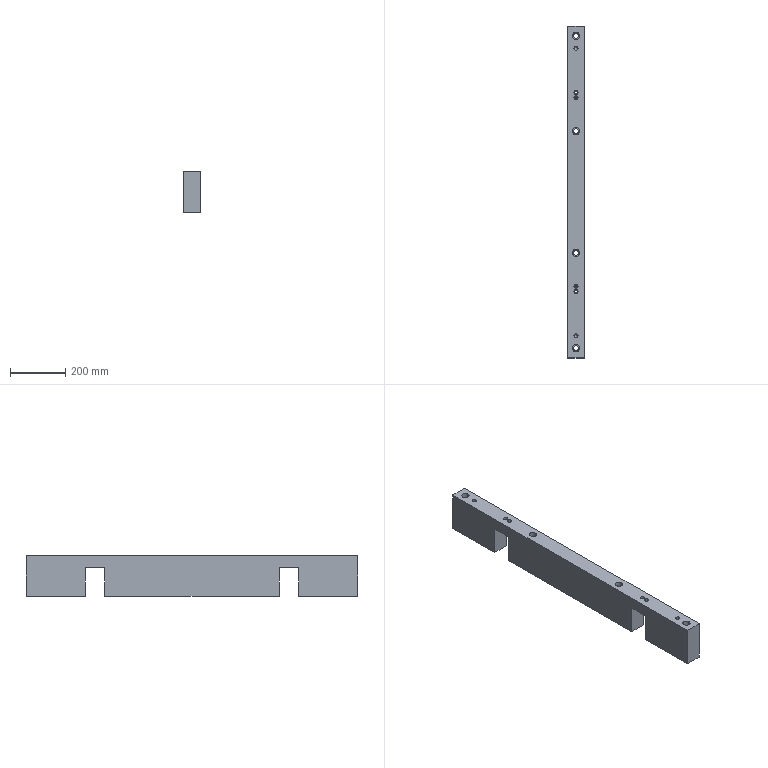Part | STEP file | lll_id2326_x_t | 1 solid | 42 faces | box 60 x 1200 x 147.5 mm | volume 9435645 mm3 | plane 22 | cylinder 18 | cone 2 | commonest cylinder face diameters 9.009 x4 14.508 x4 18.009 x4 26.008 x4 14.506 x2
STEP:
#1=CARTESIAN_POINT('',(2957.254,-340.,370.));
#2=VERTEX_POINT('',#1);
#3=CARTESIAN_POINT('',(2950.,-340.,370.));
#4=DIRECTION('',(0.,0.,-1.));
#5=DIRECTION('',(1.,0.,0.));
#6=AXIS2_PLACEMENT_3D('',#3,#4,#5);
#7=CIRCLE('',#6,7.254);
#8=EDGE_CURVE('',#2,#2,#7,.T.);
#9=ORIENTED_EDGE('',*,*,#8,.T.);
#10=EDGE_LOOP('',(#9));
#11=FACE_BOUND('',#10,.T.);
#12=CARTESIAN_POINT('',(2957.254,-360.,370.));
#13=VERTEX_POINT('',#12);
#14=CARTESIAN_POINT('',(2950.,-360.,370.));
#15=DIRECTION('',(0.,0.,-1.));
#16=DIRECTION('',(1.,0.,0.));
#17=AXIS2_PLACEMENT_3D('',#14,#15,#16);
#18=CIRCLE('',#17,7.254);
#19=EDGE_CURVE('',#13,#13,#18,.T.);
#20=ORIENTED_EDGE('',*,*,#19,.T.);
#21=EDGE_LOOP('',(#20));
#22=FACE_BOUND('',#21,.T.);
#23=CARTESIAN_POINT('',(2957.254,340.,370.));
#24=VERTEX_POINT('',#23);
#25=CARTESIAN_POINT('',(2950.,340.,370.));
#26=DIRECTION('',(0.,0.,-1.));
#27=DIRECTION('',(1.,0.,0.));
#28=AXIS2_PLACEMENT_3D('',#25,#26,#27);
#29=CIRCLE('',#28,7.254);
#30=EDGE_CURVE('',#24,#24,#29,.T.);
#31=ORIENTED_EDGE('',*,*,#30,.T.);
#32=EDGE_LOOP('',(#31));
#33=FACE_BOUND('',#32,.T.);
#34=CARTESIAN_POINT('',(2957.254,360.,370.));
#35=VERTEX_POINT('',#34);
#36=CARTESIAN_POINT('',(2950.,360.,370.));
#37=DIRECTION('',(0.,0.,-1.));
#38=DIRECTION('',(1.,0.,0.));
#39=AXIS2_PLACEMENT_3D('',#36,#37,#38);
#40=CIRCLE('',#39,7.254);
#41=EDGE_CURVE('',#35,#35,#40,.T.);
#42=ORIENTED_EDGE('',*,*,#41,.T.);
#43=EDGE_LOOP('',(#42));
#44=FACE_BOUND('',#43,.T.);
#45=CARTESIAN_POINT('',(2963.004,220.,370.));
#46=VERTEX_POINT('',#45);
#47=CARTESIAN_POINT('',(2950.,220.,370.));
#48=DIRECTION('',(0.,0.,1.));
#49=DIRECTION('',(1.,0.,0.));
#50=AXIS2_PLACEMENT_3D('',#47,#48,#49);
#51=CIRCLE('',#50,13.004);
#52=EDGE_CURVE('',#46,#46,#51,.T.);
#53=ORIENTED_EDGE('',*,*,#52,.F.);
#54=EDGE_LOOP('',(#53));
#55=FACE_BOUND('',#54,.T.);
#56=CARTESIAN_POINT('',(2963.004,-220.,370.));
#57=VERTEX_POINT('',#56);
#58=CARTESIAN_POINT('',(2950.,-220.,370.));
#59=DIRECTION('',(0.,0.,-1.));
#60=DIRECTION('',(1.,0.,0.));
#61=AXIS2_PLACEMENT_3D('',#58,#59,#60);
#62=CIRCLE('',#61,13.004);
#63=EDGE_CURVE('',#57,#57,#62,.T.);
#64=ORIENTED_EDGE('',*,*,#63,.T.);
#65=EDGE_LOOP('',(#64));
#66=FACE_BOUND('',#65,.T.);
#67=CARTESIAN_POINT('',(2963.004,-565.,370.));
#68=VERTEX_POINT('',#67);
#69=CARTESIAN_POINT('',(2950.,-565.,370.));
#70=DIRECTION('',(0.,0.,-1.));
#71=DIRECTION('',(1.,0.,0.));
#72=AXIS2_PLACEMENT_3D('',#69,#70,#71);
#73=CIRCLE('',#72,13.004);
#74=EDGE_CURVE('',#68,#68,#73,.T.);
#75=ORIENTED_EDGE('',*,*,#74,.T.);
#76=EDGE_LOOP('',(#75));
#77=FACE_BOUND('',#76,.T.);
#78=CARTESIAN_POINT('',(2980.,600.,370.));
#79=VERTEX_POINT('',#78);
#80=CARTESIAN_POINT('',(2920.,600.,370.));
#81=VERTEX_POINT('',#80);
#82=CARTESIAN_POINT('',(6890.,600.,370.));
#83=DIRECTION('',(-1.,0.,0.));
#84=VECTOR('',#83,1.);
#85=LINE('',#82,#84);
#86=EDGE_CURVE('',#79,#81,#85,.T.);
#87=ORIENTED_EDGE('',*,*,#86,.T.);
#88=CARTESIAN_POINT('',(2920.,-600.,370.));
#89=VERTEX_POINT('',#88);
#90=CARTESIAN_POINT('',(2920.,600.,370.));
#91=DIRECTION('',(0.,-1.,0.));
#92=VECTOR('',#91,1.);
#93=LINE('',#90,#92);
#94=EDGE_CURVE('',#81,#89,#93,.T.);
#95=ORIENTED_EDGE('',*,*,#94,.T.);
#96=CARTESIAN_POINT('',(2980.,-600.,370.));
#97=VERTEX_POINT('',#96);
#98=CARTESIAN_POINT('',(2920.,-600.,370.));
#99=DIRECTION('',(1.,0.,0.));
#100=VECTOR('',#99,1.);
#101=LINE('',#98,#100);
#102=EDGE_CURVE('',#89,#97,#101,.T.);
#103=ORIENTED_EDGE('',*,*,#102,.T.);
#104=CARTESIAN_POINT('',(2980.,1.,370.));
#105=DIRECTION('',(0.,1.,0.));
#106=VECTOR('',#105,1.);
#107=LINE('',#104,#106);
#108=EDGE_CURVE('',#97,#79,#107,.T.);
#109=ORIENTED_EDGE('',*,*,#108,.T.);
#110=EDGE_LOOP('',(#87,#95,#103,#109));
#111=FACE_BOUND('',#110,.T.);
#112=CARTESIAN_POINT('',(2963.004,565.,370.));
#113=VERTEX_POINT('',#112);
#114=CARTESIAN_POINT('',(2950.,565.,370.));
#115=DIRECTION('',(0.,0.,1.));
#116=DIRECTION('',(1.,0.,0.));
#117=AXIS2_PLACEMENT_3D('',#114,#115,#116);
#118=CIRCLE('',#117,13.004);
#119=EDGE_CURVE('',#113,#113,#118,.T.);
#120=ORIENTED_EDGE('',*,*,#119,.F.);
#121=EDGE_LOOP('',(#120));
#122=FACE_BOUND('',#121,.T.);
#123=CARTESIAN_POINT('',(2957.253,-520.,370.));
#124=VERTEX_POINT('',#123);
#125=CARTESIAN_POINT('',(2950.,-520.,370.));
#126=DIRECTION('',(0.,0.,-1.));
#127=DIRECTION('',(1.,0.,0.));
#128=AXIS2_PLACEMENT_3D('',#125,#126,#127);
#129=CIRCLE('',#128,7.253);
#130=EDGE_CURVE('',#124,#124,#129,.T.);
#131=ORIENTED_EDGE('',*,*,#130,.T.);
#132=EDGE_LOOP('',(#131));
#133=FACE_BOUND('',#132,.T.);
#134=CARTESIAN_POINT('',(2957.253,520.,370.));
#135=VERTEX_POINT('',#134);
#136=CARTESIAN_POINT('',(2950.,520.,370.));
#137=DIRECTION('',(0.,0.,1.));
#138=DIRECTION('',(1.,0.,0.));
#139=AXIS2_PLACEMENT_3D('',#136,#137,#138);
#140=CIRCLE('',#139,7.253);
#141=EDGE_CURVE('',#135,#135,#140,.T.);
#142=ORIENTED_EDGE('',*,*,#141,.F.);
#143=EDGE_LOOP('',(#142));
#144=FACE_BOUND('',#143,.T.);
#145=CARTESIAN_POINT('',(733.685,1.,370.));
#146=DIRECTION('',(0.,0.,-1.));
#147=DIRECTION('',(1.,0.,0.));
#148=AXIS2_PLACEMENT_3D('',#145,#146,#147);
#149=PLANE('',#148);
#150=ADVANCED_FACE('',(#11,#22,#33,#44,#55,#66,#77,#111,#122,#133,#144),#149,.F.);
#151=CARTESIAN_POINT('',(2980.,315.249,222.5));
#152=VERTEX_POINT('',#151);
#153=CARTESIAN_POINT('',(2920.,315.249,222.5));
#154=VERTEX_POINT('',#153);
#155=CARTESIAN_POINT('',(733.685,315.249,222.5));
#156=DIRECTION('',(-1.,0.,0.));
#157=VECTOR('',#156,1.);
#158=LINE('',#155,#157);
#159=EDGE_CURVE('',#152,#154,#158,.T.);
#160=ORIENTED_EDGE('',*,*,#159,.F.);
#161=CARTESIAN_POINT('',(2980.,-315.249,222.5));
#162=VERTEX_POINT('',#161);
#163=CARTESIAN_POINT('',(2980.,1.,222.5));
#164=DIRECTION('',(0.,-1.,0.));
#165=VECTOR('',#164,1.);
#166=LINE('',#163,#165);
#167=EDGE_CURVE('',#152,#162,#166,.T.);
#168=ORIENTED_EDGE('',*,*,#167,.T.);
#169=CARTESIAN_POINT('',(2920.,-315.249,222.5));
#170=VERTEX_POINT('',#169);
#171=CARTESIAN_POINT('',(733.685,-315.249,222.5));
#172=DIRECTION('',(1.,0.,0.));
#173=VECTOR('',#172,1.);
#174=LINE('',#171,#173);
#175=EDGE_CURVE('',#170,#162,#174,.T.);
#176=ORIENTED_EDGE('',*,*,#175,.F.);
#177=CARTESIAN_POINT('',(2920.,600.,222.5));
#178=DIRECTION('',(0.,-1.,0.));
#179=VECTOR('',#178,1.);
#180=LINE('',#177,#179);
#181=EDGE_CURVE('',#154,#170,#180,.T.);
#182=ORIENTED_EDGE('',*,*,#181,.F.);
#183=EDGE_LOOP('',(#160,#168,#176,#182));
#184=FACE_BOUND('',#183,.T.);
#185=CARTESIAN_POINT('',(2959.005,220.,222.5));
#186=VERTEX_POINT('',#185);
#187=CARTESIAN_POINT('',(2950.,220.,222.5));
#188=DIRECTION('',(0.,0.,-1.));
#189=DIRECTION('',(1.,0.,0.));
#190=AXIS2_PLACEMENT_3D('',#187,#188,#189);
#191=CIRCLE('',#190,9.005);
#192=EDGE_CURVE('',#186,#186,#191,.T.);
#193=ORIENTED_EDGE('',*,*,#192,.F.);
#194=EDGE_LOOP('',(#193));
#195=FACE_BOUND('',#194,.T.);
#196=CARTESIAN_POINT('',(2959.005,-220.,222.5));
#197=VERTEX_POINT('',#196);
#198=CARTESIAN_POINT('',(2950.,-220.,222.5));
#199=DIRECTION('',(0.,0.,1.));
#200=DIRECTION('',(1.,0.,0.));
#201=AXIS2_PLACEMENT_3D('',#198,#199,#200);
#202=CIRCLE('',#201,9.005);
#203=EDGE_CURVE('',#197,#197,#202,.T.);
#204=ORIENTED_EDGE('',*,*,#203,.T.);
#205=EDGE_LOOP('',(#204));
#206=FACE_BOUND('',#205,.T.);
#207=CARTESIAN_POINT('',(733.685,1.,222.5));
#208=DIRECTION('',(0.,0.,-1.));
#209=DIRECTION('',(1.,0.,0.));
#210=AXIS2_PLACEMENT_3D('',#207,#208,#209);
#211=PLANE('',#210);
#212=ADVANCED_FACE('',(#184,#195,#206),#211,.T.);
#213=CARTESIAN_POINT('',(2920.,385.249,222.5));
#214=VERTEX_POINT('',#213);
#215=CARTESIAN_POINT('',(2980.,385.249,222.5));
#216=VERTEX_POINT('',#215);
#217=CARTESIAN_POINT('',(733.685,385.249,222.5));
#218=DIRECTION('',(1.,0.,0.));
#219=VECTOR('',#218,1.);
#220=LINE('',#217,#219);
#221=EDGE_CURVE('',#214,#216,#220,.T.);
#222=ORIENTED_EDGE('',*,*,#221,.F.);
#223=CARTESIAN_POINT('',(2920.,600.,222.5));
#224=VERTEX_POINT('',#223);
#225=CARTESIAN_POINT('',(2920.,600.,222.5));
#226=DIRECTION('',(0.,-1.,0.));
#227=VECTOR('',#226,1.);
#228=LINE('',#225,#227);
#229=EDGE_CURVE('',#224,#214,#228,.T.);
#230=ORIENTED_EDGE('',*,*,#229,.F.);
#231=CARTESIAN_POINT('',(2980.,600.,222.5));
#232=VERTEX_POINT('',#231);
#233=CARTESIAN_POINT('',(6890.,600.,222.5));
#234=DIRECTION('',(-1.,0.,0.));
#235=VECTOR('',#234,1.);
#236=LINE('',#233,#235);
#237=EDGE_CURVE('',#232,#224,#236,.T.);
#238=ORIENTED_EDGE('',*,*,#237,.F.);
#239=CARTESIAN_POINT('',(2980.,1.,222.5));
#240=DIRECTION('',(0.,-1.,0.));
#241=VECTOR('',#240,1.);
#242=LINE('',#239,#241);
#243=EDGE_CURVE('',#232,#216,#242,.T.);
#244=ORIENTED_EDGE('',*,*,#243,.T.);
#245=EDGE_LOOP('',(#222,#230,#238,#244));
#246=FACE_BOUND('',#245,.T.);
#247=CARTESIAN_POINT('',(2959.005,565.,222.5));
#248=VERTEX_POINT('',#247);
#249=CARTESIAN_POINT('',(2950.,565.,222.5));
#250=DIRECTION('',(0.,0.,-1.));
#251=DIRECTION('',(1.,0.,0.));
#252=AXIS2_PLACEMENT_3D('',#249,#250,#251);
#253=CIRCLE('',#252,9.005);
#254=EDGE_CURVE('',#248,#248,#253,.T.);
#255=ORIENTED_EDGE('',*,*,#254,.F.);
#256=EDGE_LOOP('',(#255));
#257=FACE_BOUND('',#256,.T.);
#258=CARTESIAN_POINT('',(733.685,1.,222.5));
#259=DIRECTION('',(0.,0.,-1.));
#260=DIRECTION('',(1.,0.,0.));
#261=AXIS2_PLACEMENT_3D('',#258,#259,#260);
#262=PLANE('',#261);
#263=ADVANCED_FACE('',(#246,#257),#262,.T.);
#264=CARTESIAN_POINT('',(2980.,-385.249,222.5));
#265=VERTEX_POINT('',#264);
#266=CARTESIAN_POINT('',(2920.,-385.249,222.5));
#267=VERTEX_POINT('',#266);
#268=CARTESIAN_POINT('',(733.685,-385.249,222.5));
#269=DIRECTION('',(-1.,0.,0.));
#270=VECTOR('',#269,1.);
#271=LINE('',#268,#270);
#272=EDGE_CURVE('',#265,#267,#271,.T.);
#273=ORIENTED_EDGE('',*,*,#272,.F.);
#274=CARTESIAN_POINT('',(2980.,-600.,222.5));
#275=VERTEX_POINT('',#274);
#276=CARTESIAN_POINT('',(2980.,1.,222.5));
#277=DIRECTION('',(0.,-1.,0.));
#278=VECTOR('',#277,1.);
#279=LINE('',#276,#278);
#280=EDGE_CURVE('',#265,#275,#279,.T.);
#281=ORIENTED_EDGE('',*,*,#280,.T.);
#282=CARTESIAN_POINT('',(2920.,-600.,222.5));
#283=VERTEX_POINT('',#282);
#284=CARTESIAN_POINT('',(2920.,-600.,222.5));
#285=DIRECTION('',(1.,0.,0.));
#286=VECTOR('',#285,1.);
#287=LINE('',#284,#286);
#288=EDGE_CURVE('',#283,#275,#287,.T.);
#289=ORIENTED_EDGE('',*,*,#288,.F.);
#290=CARTESIAN_POINT('',(2920.,600.,222.5));
#291=DIRECTION('',(0.,-1.,0.));
#292=VECTOR('',#291,1.);
#293=LINE('',#290,#292);
#294=EDGE_CURVE('',#267,#283,#293,.T.);
#295=ORIENTED_EDGE('',*,*,#294,.F.);
#296=EDGE_LOOP('',(#273,#281,#289,#295));
#297=FACE_BOUND('',#296,.T.);
#298=CARTESIAN_POINT('',(2959.005,-565.,222.5));
#299=VERTEX_POINT('',#298);
#300=CARTESIAN_POINT('',(2950.,-565.,222.5));
#301=DIRECTION('',(0.,0.,1.));
#302=DIRECTION('',(1.,0.,0.));
#303=AXIS2_PLACEMENT_3D('',#300,#301,#302);
#304=CIRCLE('',#303,9.005);
#305=EDGE_CURVE('',#299,#299,#304,.T.);
#306=ORIENTED_EDGE('',*,*,#305,.T.);
#307=EDGE_LOOP('',(#306));
#308=FACE_BOUND('',#307,.T.);
#309=CARTESIAN_POINT('',(733.685,1.,222.5));
#310=DIRECTION('',(0.,0.,-1.));
#311=DIRECTION('',(1.,0.,0.));
#312=AXIS2_PLACEMENT_3D('',#309,#310,#311);
#313=PLANE('',#312);
#314=ADVANCED_FACE('',(#297,#308),#313,.T.);
#315=CARTESIAN_POINT('',(2920.,315.249,326.5));
#316=VERTEX_POINT('',#315);
#317=CARTESIAN_POINT('',(2920.,315.249,310.));
#318=DIRECTION('',(0.,0.,1.));
#319=VECTOR('',#318,1.);
#320=LINE('',#317,#319);
#321=EDGE_CURVE('',#154,#316,#320,.T.);
#322=ORIENTED_EDGE('',*,*,#321,.F.);
#323=ORIENTED_EDGE('',*,*,#181,.T.);
#324=CARTESIAN_POINT('',(2920.,-315.249,326.5));
#325=VERTEX_POINT('',#324);
#326=CARTESIAN_POINT('',(2920.,-315.249,310.));
#327=DIRECTION('',(0.,0.,-1.));
#328=VECTOR('',#327,1.);
#329=LINE('',#326,#328);
#330=EDGE_CURVE('',#325,#170,#329,.T.);
#331=ORIENTED_EDGE('',*,*,#330,.F.);
#332=CARTESIAN_POINT('',(2920.,-385.249,326.5));
#333=VERTEX_POINT('',#332);
#334=CARTESIAN_POINT('',(2920.,600.,326.5));
#335=DIRECTION('',(0.,1.,0.));
#336=VECTOR('',#335,1.);
#337=LINE('',#334,#336);
#338=EDGE_CURVE('',#333,#325,#337,.T.);
#339=ORIENTED_EDGE('',*,*,#338,.F.);
#340=CARTESIAN_POINT('',(2920.,-385.249,310.));
#341=DIRECTION('',(0.,0.,1.));
#342=VECTOR('',#341,1.);
#343=LINE('',#340,#342);
#344=EDGE_CURVE('',#267,#333,#343,.T.);
#345=ORIENTED_EDGE('',*,*,#344,.F.);
#346=ORIENTED_EDGE('',*,*,#294,.T.);
#347=CARTESIAN_POINT('',(2920.,-600.,310.));
#348=DIRECTION('',(0.,0.,-1.));
#349=VECTOR('',#348,1.);
#350=LINE('',#347,#349);
#351=EDGE_CURVE('',#89,#283,#350,.T.);
#352=ORIENTED_EDGE('',*,*,#351,.F.);
#353=ORIENTED_EDGE('',*,*,#94,.F.);
#354=CARTESIAN_POINT('',(2920.,600.,310.));
#355=DIRECTION('',(0.,0.,-1.));
#356=VECTOR('',#355,1.);
#357=LINE('',#354,#356);
#358=EDGE_CURVE('',#81,#224,#357,.T.);
#359=ORIENTED_EDGE('',*,*,#358,.T.);
#360=ORIENTED_EDGE('',*,*,#229,.T.);
#361=CARTESIAN_POINT('',(2920.,385.249,326.5));
#362=VERTEX_POINT('',#361);
#363=CARTESIAN_POINT('',(2920.,385.249,310.));
#364=DIRECTION('',(0.,0.,-1.));
#365=VECTOR('',#364,1.);
#366=LINE('',#363,#365);
#367=EDGE_CURVE('',#362,#214,#366,.T.);
#368=ORIENTED_EDGE('',*,*,#367,.F.);
#369=CARTESIAN_POINT('',(2920.,600.,326.5));
#370=DIRECTION('',(0.,1.,0.));
#371=VECTOR('',#370,1.);
#372=LINE('',#369,#371);
#373=EDGE_CURVE('',#316,#362,#372,.T.);
#374=ORIENTED_EDGE('',*,*,#373,.F.);
#375=EDGE_LOOP('',(#322,#323,#331,#339,#345,#346,#352,#353,#359,#360,#368,#374));
#376=FACE_OUTER_BOUND('',#375,.T.);
#377=CARTESIAN_POINT('',(2920.,600.,310.));
#378=DIRECTION('',(-1.,0.,0.));
#379=DIRECTION('',(0.,0.,-1.));
#380=AXIS2_PLACEMENT_3D('',#377,#378,#379);
#381=PLANE('',#380);
#382=ADVANCED_FACE('',(#376),#381,.T.);
#383=CARTESIAN_POINT('',(2980.,-600.,310.));
#384=DIRECTION('',(0.,0.,-1.));
#385=VECTOR('',#384,1.);
#386=LINE('',#383,#385);
#387=EDGE_CURVE('',#97,#275,#386,.T.);
#388=ORIENTED_EDGE('',*,*,#387,.F.);
#389=ORIENTED_EDGE('',*,*,#102,.F.);
#390=ORIENTED_EDGE('',*,*,#351,.T.);
#391=ORIENTED_EDGE('',*,*,#288,.T.);
#392=EDGE_LOOP('',(#388,#389,#390,#391));
#393=FACE_OUTER_BOUND('',#392,.T.);
#394=CARTESIAN_POINT('',(2920.,-600.,310.));
#395=DIRECTION('',(0.,-1.,0.));
#396=DIRECTION('',(0.,0.,-1.));
#397=AXIS2_PLACEMENT_3D('',#394,#395,#396);
#398=PLANE('',#397);
#399=ADVANCED_FACE('',(#393),#398,.T.);
#400=CARTESIAN_POINT('',(2980.,600.,310.));
#401=DIRECTION('',(0.,0.,1.));
#402=VECTOR('',#401,1.);
#403=LINE('',#400,#402);
#404=EDGE_CURVE('',#232,#79,#403,.T.);
#405=ORIENTED_EDGE('',*,*,#404,.F.);
#406=ORIENTED_EDGE('',*,*,#237,.T.);
#407=ORIENTED_EDGE('',*,*,#358,.F.);
#408=ORIENTED_EDGE('',*,*,#86,.F.);
#409=EDGE_LOOP('',(#405,#406,#407,#408));
#410=FACE_OUTER_BOUND('',#409,.T.);
#411=CARTESIAN_POINT('',(6890.,600.,310.));
#412=DIRECTION('',(0.,1.,0.));
#413=DIRECTION('',(0.,0.,1.));
#414=AXIS2_PLACEMENT_3D('',#411,#412,#413);
#415=PLANE('',#414);
#416=ADVANCED_FACE('',(#410),#415,.T.);
#417=ORIENTED_EDGE('',*,*,#167,.F.);
#418=CARTESIAN_POINT('',(2980.,315.249,326.5));
#419=VERTEX_POINT('',#418);
#420=CARTESIAN_POINT('',(2980.,315.249,241.25));
#421=DIRECTION('',(0.,0.,1.));
#422=VECTOR('',#421,1.);
#423=LINE('',#420,#422);
#424=EDGE_CURVE('',#152,#419,#423,.T.);
#425=ORIENTED_EDGE('',*,*,#424,.T.);
#426=CARTESIAN_POINT('',(2980.,385.249,326.5));
#427=VERTEX_POINT('',#426);
#428=CARTESIAN_POINT('',(2980.,0.,326.5));
#429=DIRECTION('',(0.,1.,0.));
#430=VECTOR('',#429,1.);
#431=LINE('',#428,#430);
#432=EDGE_CURVE('',#419,#427,#431,.T.);
#433=ORIENTED_EDGE('',*,*,#432,.T.);
#434=CARTESIAN_POINT('',(2980.,385.249,241.25));
#435=DIRECTION('',(0.,0.,-1.));
#436=VECTOR('',#435,1.);
#437=LINE('',#434,#436);
#438=EDGE_CURVE('',#427,#216,#437,.T.);
#439=ORIENTED_EDGE('',*,*,#438,.T.);
#440=ORIENTED_EDGE('',*,*,#243,.F.);
#441=ORIENTED_EDGE('',*,*,#404,.T.);
#442=ORIENTED_EDGE('',*,*,#108,.F.);
#443=ORIENTED_EDGE('',*,*,#387,.T.);
#444=ORIENTED_EDGE('',*,*,#280,.F.);
#445=CARTESIAN_POINT('',(2980.,-385.249,326.5));
#446=VERTEX_POINT('',#445);
#447=CARTESIAN_POINT('',(2980.,-385.249,241.25));
#448=DIRECTION('',(0.,0.,1.));
#449=VECTOR('',#448,1.);
#450=LINE('',#447,#449);
#451=EDGE_CURVE('',#265,#446,#450,.T.);
#452=ORIENTED_EDGE('',*,*,#451,.T.);
#453=CARTESIAN_POINT('',(2980.,-315.249,326.5));
#454=VERTEX_POINT('',#453);
#455=CARTESIAN_POINT('',(2980.,0.,326.5));
#456=DIRECTION('',(0.,1.,0.));
#457=VECTOR('',#456,1.);
#458=LINE('',#455,#457);
#459=EDGE_CURVE('',#446,#454,#458,.T.);
#460=ORIENTED_EDGE('',*,*,#459,.T.);
#461=CARTESIAN_POINT('',(2980.,-315.249,241.25));
#462=DIRECTION('',(0.,0.,-1.));
#463=VECTOR('',#462,1.);
#464=LINE('',#461,#463);
#465=EDGE_CURVE('',#454,#162,#464,.T.);
#466=ORIENTED_EDGE('',*,*,#465,.T.);
#467=EDGE_LOOP('',(#417,#425,#433,#439,#440,#441,#442,#443,#444,#452,#460,#466));
#468=FACE_OUTER_BOUND('',#467,.T.);
#469=CARTESIAN_POINT('',(2980.,0.,241.25));
#470=DIRECTION('',(-1.,0.,0.));
#471=DIRECTION('',(0.,0.,-1.));
#472=AXIS2_PLACEMENT_3D('',#469,#470,#471);
#473=PLANE('',#472);
#474=ADVANCED_FACE('',(#468),#473,.F.);
#475=CARTESIAN_POINT('',(2940.995,-565.,251.));
#476=VERTEX_POINT('',#475);
#477=CARTESIAN_POINT('',(2950.,-565.,251.));
#478=DIRECTION('',(0.,0.,-1.));
#479=DIRECTION('',(-1.,0.,0.));
#480=AXIS2_PLACEMENT_3D('',#477,#478,#479);
#481=CIRCLE('',#480,9.005);
#482=EDGE_CURVE('',#476,#476,#481,.T.);
#483=ORIENTED_EDGE('',*,*,#482,.F.);
#484=EDGE_LOOP('',(#483));
#485=FACE_BOUND('',#484,.T.);
#486=ORIENTED_EDGE('',*,*,#305,.F.);
#487=EDGE_LOOP('',(#486));
#488=FACE_BOUND('',#487,.T.);
#489=CARTESIAN_POINT('',(2950.,-565.,370.));
#490=DIRECTION('',(0.,0.,-1.));
#491=DIRECTION('',(1.,0.,0.));
#492=AXIS2_PLACEMENT_3D('',#489,#490,#491);
#493=CYLINDRICAL_SURFACE('',#492,9.005);
#494=ADVANCED_FACE('',(#485,#488),#493,.F.);
#495=ORIENTED_EDGE('',*,*,#482,.T.);
#496=EDGE_LOOP('',(#495));
#497=FACE_BOUND('',#496,.T.);
#498=CARTESIAN_POINT('',(2963.004,-565.,251.));
#499=VERTEX_POINT('',#498);
#500=CARTESIAN_POINT('',(2950.,-565.,251.));
#501=DIRECTION('',(0.,0.,-1.));
#502=DIRECTION('',(1.,0.,0.));
#503=AXIS2_PLACEMENT_3D('',#500,#501,#502);
#504=CIRCLE('',#503,13.004);
#505=EDGE_CURVE('',#499,#499,#504,.T.);
#506=ORIENTED_EDGE('',*,*,#505,.F.);
#507=EDGE_LOOP('',(#506));
#508=FACE_BOUND('',#507,.T.);
#509=CARTESIAN_POINT('',(2950.,-565.,251.));
#510=DIRECTION('',(0.,0.,-1.));
#511=DIRECTION('',(-1.,0.,0.));
#512=AXIS2_PLACEMENT_3D('',#509,#510,#511);
#513=PLANE('',#512);
#514=ADVANCED_FACE('',(#497,#508),#513,.F.);
#515=ORIENTED_EDGE('',*,*,#505,.T.);
#516=EDGE_LOOP('',(#515));
#517=FACE_BOUND('',#516,.T.);
#518=ORIENTED_EDGE('',*,*,#74,.F.);
#519=EDGE_LOOP('',(#518));
#520=FACE_BOUND('',#519,.T.);
#521=CARTESIAN_POINT('',(2950.,-565.,370.));
#522=DIRECTION('',(0.,0.,-1.));
#523=DIRECTION('',(1.,0.,0.));
#524=AXIS2_PLACEMENT_3D('',#521,#522,#523);
#525=CYLINDRICAL_SURFACE('',#524,13.004);
#526=ADVANCED_FACE('',(#517,#520),#525,.F.);
#527=CARTESIAN_POINT('',(2940.995,-220.,251.));
#528=VERTEX_POINT('',#527);
#529=CARTESIAN_POINT('',(2950.,-220.,251.));
#530=DIRECTION('',(0.,0.,-1.));
#531=DIRECTION('',(-1.,0.,0.));
#532=AXIS2_PLACEMENT_3D('',#529,#530,#531);
#533=CIRCLE('',#532,9.005);
#534=EDGE_CURVE('',#528,#528,#533,.T.);
#535=ORIENTED_EDGE('',*,*,#534,.F.);
#536=EDGE_LOOP('',(#535));
#537=FACE_BOUND('',#536,.T.);
#538=ORIENTED_EDGE('',*,*,#203,.F.);
#539=EDGE_LOOP('',(#538));
#540=FACE_BOUND('',#539,.T.);
#541=CARTESIAN_POINT('',(2950.,-220.,370.));
#542=DIRECTION('',(0.,0.,-1.));
#543=DIRECTION('',(1.,0.,0.));
#544=AXIS2_PLACEMENT_3D('',#541,#542,#543);
#545=CYLINDRICAL_SURFACE('',#544,9.005);
#546=ADVANCED_FACE('',(#537,#540),#545,.F.);
#547=ORIENTED_EDGE('',*,*,#534,.T.);
#548=EDGE_LOOP('',(#547));
#549=FACE_BOUND('',#548,.T.);
#550=CARTESIAN_POINT('',(2963.004,-220.,251.));
#551=VERTEX_POINT('',#550);
#552=CARTESIAN_POINT('',(2950.,-220.,251.));
#553=DIRECTION('',(0.,0.,-1.));
#554=DIRECTION('',(1.,0.,0.));
#555=AXIS2_PLACEMENT_3D('',#552,#553,#554);
#556=CIRCLE('',#555,13.004);
#557=EDGE_CURVE('',#551,#551,#556,.T.);
#558=ORIENTED_EDGE('',*,*,#557,.F.);
#559=EDGE_LOOP('',(#558));
#560=FACE_BOUND('',#559,.T.);
#561=CARTESIAN_POINT('',(2950.,-220.,251.));
#562=DIRECTION('',(0.,0.,-1.));
#563=DIRECTION('',(-1.,0.,0.));
#564=AXIS2_PLACEMENT_3D('',#561,#562,#563);
#565=PLANE('',#564);
#566=ADVANCED_FACE('',(#549,#560),#565,.F.);
#567=ORIENTED_EDGE('',*,*,#557,.T.);
#568=EDGE_LOOP('',(#567));
#569=FACE_BOUND('',#568,.T.);
#570=ORIENTED_EDGE('',*,*,#63,.F.);
#571=EDGE_LOOP('',(#570));
#572=FACE_BOUND('',#571,.T.);
#573=CARTESIAN_POINT('',(2950.,-220.,370.));
#574=DIRECTION('',(0.,0.,-1.));
#575=DIRECTION('',(1.,0.,0.));
#576=AXIS2_PLACEMENT_3D('',#573,#574,#575);
#577=CYLINDRICAL_SURFACE('',#576,13.004);
#578=ADVANCED_FACE('',(#569,#572),#577,.F.);
#579=CARTESIAN_POINT('',(2940.995,220.,251.));
#580=VERTEX_POINT('',#579);
#581=CARTESIAN_POINT('',(2950.,220.,251.));
#582=DIRECTION('',(0.,0.,1.));
#583=DIRECTION('',(-1.,0.,0.));
#584=AXIS2_PLACEMENT_3D('',#581,#582,#583);
#585=CIRCLE('',#584,9.005);
#586=EDGE_CURVE('',#580,#580,#585,.T.);
#587=ORIENTED_EDGE('',*,*,#586,.T.);
#588=EDGE_LOOP('',(#587));
#589=FACE_BOUND('',#588,.T.);
#590=ORIENTED_EDGE('',*,*,#192,.T.);
#591=EDGE_LOOP('',(#590));
#592=FACE_BOUND('',#591,.T.);
#593=CARTESIAN_POINT('',(2950.,220.,370.));
#594=DIRECTION('',(0.,0.,-1.));
#595=DIRECTION('',(1.,0.,0.));
#596=AXIS2_PLACEMENT_3D('',#593,#594,#595);
#597=CYLINDRICAL_SURFACE('',#596,9.005);
#598=ADVANCED_FACE('',(#589,#592),#597,.F.);
#599=ORIENTED_EDGE('',*,*,#586,.F.);
#600=EDGE_LOOP('',(#599));
#601=FACE_BOUND('',#600,.T.);
#602=CARTESIAN_POINT('',(2963.004,220.,251.));
#603=VERTEX_POINT('',#602);
#604=CARTESIAN_POINT('',(2950.,220.,251.));
#605=DIRECTION('',(0.,0.,1.));
#606=DIRECTION('',(1.,0.,0.));
#607=AXIS2_PLACEMENT_3D('',#604,#605,#606);
#608=CIRCLE('',#607,13.004);
#609=EDGE_CURVE('',#603,#603,#608,.T.);
#610=ORIENTED_EDGE('',*,*,#609,.T.);
#611=EDGE_LOOP('',(#610));
#612=FACE_BOUND('',#611,.T.);
#613=CARTESIAN_POINT('',(2950.,220.,251.));
#614=DIRECTION('',(0.,0.,-1.));
#615=DIRECTION('',(-1.,0.,0.));
#616=AXIS2_PLACEMENT_3D('',#613,#614,#615);
#617=PLANE('',#616);
#618=ADVANCED_FACE('',(#601,#612),#617,.F.);
#619=ORIENTED_EDGE('',*,*,#609,.F.);
#620=EDGE_LOOP('',(#619));
#621=FACE_BOUND('',#620,.T.);
#622=ORIENTED_EDGE('',*,*,#52,.T.);
#623=EDGE_LOOP('',(#622));
#624=FACE_BOUND('',#623,.T.);
#625=CARTESIAN_POINT('',(2950.,220.,370.));
#626=DIRECTION('',(0.,0.,-1.));
#627=DIRECTION('',(1.,0.,0.));
#628=AXIS2_PLACEMENT_3D('',#625,#626,#627);
#629=CYLINDRICAL_SURFACE('',#628,13.004);
#630=ADVANCED_FACE('',(#621,#624),#629,.F.);
#631=CARTESIAN_POINT('',(2940.995,565.,251.));
#632=VERTEX_POINT('',#631);
#633=CARTESIAN_POINT('',(2950.,565.,251.));
#634=DIRECTION('',(0.,0.,1.));
#635=DIRECTION('',(-1.,0.,0.));
#636=AXIS2_PLACEMENT_3D('',#633,#634,#635);
#637=CIRCLE('',#636,9.005);
#638=EDGE_CURVE('',#632,#632,#637,.T.);
#639=ORIENTED_EDGE('',*,*,#638,.T.);
#640=EDGE_LOOP('',(#639));
#641=FACE_BOUND('',#640,.T.);
#642=ORIENTED_EDGE('',*,*,#254,.T.);
#643=EDGE_LOOP('',(#642));
#644=FACE_BOUND('',#643,.T.);
#645=CARTESIAN_POINT('',(2950.,565.,370.));
#646=DIRECTION('',(0.,0.,-1.));
#647=DIRECTION('',(1.,0.,0.));
#648=AXIS2_PLACEMENT_3D('',#645,#646,#647);
#649=CYLINDRICAL_SURFACE('',#648,9.005);
#650=ADVANCED_FACE('',(#641,#644),#649,.F.);
#651=ORIENTED_EDGE('',*,*,#638,.F.);
#652=EDGE_LOOP('',(#651));
#653=FACE_BOUND('',#652,.T.);
#654=CARTESIAN_POINT('',(2963.004,565.,251.));
#655=VERTEX_POINT('',#654);
#656=CARTESIAN_POINT('',(2950.,565.,251.));
#657=DIRECTION('',(0.,0.,1.));
#658=DIRECTION('',(1.,0.,0.));
#659=AXIS2_PLACEMENT_3D('',#656,#657,#658);
#660=CIRCLE('',#659,13.004);
#661=EDGE_CURVE('',#655,#655,#660,.T.);
#662=ORIENTED_EDGE('',*,*,#661,.T.);
#663=EDGE_LOOP('',(#662));
#664=FACE_BOUND('',#663,.T.);
#665=CARTESIAN_POINT('',(2950.,565.,251.));
#666=DIRECTION('',(0.,0.,-1.));
#667=DIRECTION('',(-1.,0.,0.));
#668=AXIS2_PLACEMENT_3D('',#665,#666,#667);
#669=PLANE('',#668);
#670=ADVANCED_FACE('',(#653,#664),#669,.F.);
#671=ORIENTED_EDGE('',*,*,#661,.F.);
#672=EDGE_LOOP('',(#671));
#673=FACE_BOUND('',#672,.T.);
#674=ORIENTED_EDGE('',*,*,#119,.T.);
#675=EDGE_LOOP('',(#674));
#676=FACE_BOUND('',#675,.T.);
#677=CARTESIAN_POINT('',(2950.,565.,370.));
#678=DIRECTION('',(0.,0.,-1.));
#679=DIRECTION('',(1.,0.,0.));
#680=AXIS2_PLACEMENT_3D('',#677,#678,#679);
#681=CYLINDRICAL_SURFACE('',#680,13.004);
#682=ADVANCED_FACE('',(#673,#676),#681,.F.);
#683=CARTESIAN_POINT('',(2954.505,-340.,326.5));
#684=VERTEX_POINT('',#683);
#685=CARTESIAN_POINT('',(2950.,-340.,326.5));
#686=DIRECTION('',(0.,0.,1.));
#687=DIRECTION('',(1.,0.,0.));
#688=AXIS2_PLACEMENT_3D('',#685,#686,#687);
#689=CIRCLE('',#688,4.505);
#690=EDGE_CURVE('',#684,#684,#689,.T.);
#691=ORIENTED_EDGE('',*,*,#690,.T.);
#692=EDGE_LOOP('',(#691));
#693=FACE_BOUND('',#692,.T.);
#694=CARTESIAN_POINT('',(2954.505,-360.,326.5));
#695=VERTEX_POINT('',#694);
#696=CARTESIAN_POINT('',(2950.,-360.,326.5));
#697=DIRECTION('',(0.,0.,1.));
#698=DIRECTION('',(1.,0.,0.));
#699=AXIS2_PLACEMENT_3D('',#696,#697,#698);
#700=CIRCLE('',#699,4.505);
#701=EDGE_CURVE('',#695,#695,#700,.T.);
#702=ORIENTED_EDGE('',*,*,#701,.T.);
#703=EDGE_LOOP('',(#702));
#704=FACE_BOUND('',#703,.T.);
#705=ORIENTED_EDGE('',*,*,#338,.T.);
#706=CARTESIAN_POINT('',(2950.,-315.249,326.5));
#707=DIRECTION('',(1.,0.,0.));
#708=VECTOR('',#707,1.);
#709=LINE('',#706,#708);
#710=EDGE_CURVE('',#325,#454,#709,.T.);
#711=ORIENTED_EDGE('',*,*,#710,.T.);
#712=ORIENTED_EDGE('',*,*,#459,.F.);
#713=CARTESIAN_POINT('',(2950.,-385.249,326.5));
#714=DIRECTION('',(-1.,0.,0.));
#715=VECTOR('',#714,1.);
#716=LINE('',#713,#715);
#717=EDGE_CURVE('',#446,#333,#716,.T.);
#718=ORIENTED_EDGE('',*,*,#717,.T.);
#719=EDGE_LOOP('',(#705,#711,#712,#718));
#720=FACE_BOUND('',#719,.T.);
#721=CARTESIAN_POINT('',(2950.,-350.249,326.5));
#722=DIRECTION('',(0.,0.,1.));
#723=DIRECTION('',(1.,0.,0.));
#724=AXIS2_PLACEMENT_3D('',#721,#722,#723);
#725=PLANE('',#724);
#726=ADVANCED_FACE('',(#693,#704,#720),#725,.F.);
#727=ORIENTED_EDGE('',*,*,#330,.T.);
#728=ORIENTED_EDGE('',*,*,#175,.T.);
#729=ORIENTED_EDGE('',*,*,#465,.F.);
#730=ORIENTED_EDGE('',*,*,#710,.F.);
#731=EDGE_LOOP('',(#727,#728,#729,#730));
#732=FACE_OUTER_BOUND('',#731,.T.);
#733=CARTESIAN_POINT('',(2950.,-315.249,76.5));
#734=DIRECTION('',(0.,1.,0.));
#735=DIRECTION('',(0.,0.,-1.));
#736=AXIS2_PLACEMENT_3D('',#733,#734,#735);
#737=PLANE('',#736);
#738=ADVANCED_FACE('',(#732),#737,.F.);
#739=ORIENTED_EDGE('',*,*,#344,.T.);
#740=ORIENTED_EDGE('',*,*,#717,.F.);
#741=ORIENTED_EDGE('',*,*,#451,.F.);
#742=ORIENTED_EDGE('',*,*,#272,.T.);
#743=EDGE_LOOP('',(#739,#740,#741,#742));
#744=FACE_OUTER_BOUND('',#743,.T.);
#745=CARTESIAN_POINT('',(2950.,-385.249,76.5));
#746=DIRECTION('',(0.,-1.,0.));
#747=DIRECTION('',(0.,0.,1.));
#748=AXIS2_PLACEMENT_3D('',#745,#746,#747);
#749=PLANE('',#748);
#750=ADVANCED_FACE('',(#744),#749,.F.);
#751=CARTESIAN_POINT('',(2954.505,340.,326.5));
#752=VERTEX_POINT('',#751);
#753=CARTESIAN_POINT('',(2950.,340.,326.5));
#754=DIRECTION('',(0.,0.,1.));
#755=DIRECTION('',(1.,0.,0.));
#756=AXIS2_PLACEMENT_3D('',#753,#754,#755);
#757=CIRCLE('',#756,4.505);
#758=EDGE_CURVE('',#752,#752,#757,.T.);
#759=ORIENTED_EDGE('',*,*,#758,.T.);
#760=EDGE_LOOP('',(#759));
#761=FACE_BOUND('',#760,.T.);
#762=CARTESIAN_POINT('',(2954.505,360.,326.5));
#763=VERTEX_POINT('',#762);
#764=CARTESIAN_POINT('',(2950.,360.,326.5));
#765=DIRECTION('',(0.,0.,1.));
#766=DIRECTION('',(1.,0.,0.));
#767=AXIS2_PLACEMENT_3D('',#764,#765,#766);
#768=CIRCLE('',#767,4.505);
#769=EDGE_CURVE('',#763,#763,#768,.T.);
#770=ORIENTED_EDGE('',*,*,#769,.T.);
#771=EDGE_LOOP('',(#770));
#772=FACE_BOUND('',#771,.T.);
#773=ORIENTED_EDGE('',*,*,#373,.T.);
#774=CARTESIAN_POINT('',(2950.,385.249,326.5));
#775=DIRECTION('',(-1.,0.,0.));
#776=VECTOR('',#775,1.);
#777=LINE('',#774,#776);
#778=EDGE_CURVE('',#427,#362,#777,.T.);
#779=ORIENTED_EDGE('',*,*,#778,.F.);
#780=ORIENTED_EDGE('',*,*,#432,.F.);
#781=CARTESIAN_POINT('',(2950.,315.249,326.5));
#782=DIRECTION('',(1.,0.,0.));
#783=VECTOR('',#782,1.);
#784=LINE('',#781,#783);
#785=EDGE_CURVE('',#316,#419,#784,.T.);
#786=ORIENTED_EDGE('',*,*,#785,.F.);
#787=EDGE_LOOP('',(#773,#779,#780,#786));
#788=FACE_BOUND('',#787,.T.);
#789=CARTESIAN_POINT('',(2950.,350.249,326.5));
#790=DIRECTION('',(0.,0.,1.));
#791=DIRECTION('',(1.,0.,0.));
#792=AXIS2_PLACEMENT_3D('',#789,#790,#791);
#793=PLANE('',#792);
#794=ADVANCED_FACE('',(#761,#772,#788),#793,.F.);
#795=ORIENTED_EDGE('',*,*,#321,.T.);
#796=ORIENTED_EDGE('',*,*,#785,.T.);
#797=ORIENTED_EDGE('',*,*,#424,.F.);
#798=ORIENTED_EDGE('',*,*,#159,.T.);
#799=EDGE_LOOP('',(#795,#796,#797,#798));
#800=FACE_OUTER_BOUND('',#799,.T.);
#801=CARTESIAN_POINT('',(2950.,315.249,76.5));
#802=DIRECTION('',(0.,-1.,0.));
#803=DIRECTION('',(0.,0.,-1.));
#804=AXIS2_PLACEMENT_3D('',#801,#802,#803);
#805=PLANE('',#804);
#806=ADVANCED_FACE('',(#800),#805,.F.);
#807=ORIENTED_EDGE('',*,*,#367,.T.);
#808=ORIENTED_EDGE('',*,*,#221,.T.);
#809=ORIENTED_EDGE('',*,*,#438,.F.);
#810=ORIENTED_EDGE('',*,*,#778,.T.);
#811=EDGE_LOOP('',(#807,#808,#809,#810));
#812=FACE_OUTER_BOUND('',#811,.T.);
#813=CARTESIAN_POINT('',(2950.,385.249,76.5));
#814=DIRECTION('',(0.,1.,0.));
#815=DIRECTION('',(0.,0.,1.));
#816=AXIS2_PLACEMENT_3D('',#813,#814,#815);
#817=PLANE('',#816);
#818=ADVANCED_FACE('',(#812),#817,.F.);
#819=CARTESIAN_POINT('',(2945.495,360.,359.));
#820=VERTEX_POINT('',#819);
#821=CARTESIAN_POINT('',(2950.,360.,359.));
#822=DIRECTION('',(0.,0.,-1.));
#823=DIRECTION('',(-1.,0.,0.));
#824=AXIS2_PLACEMENT_3D('',#821,#822,#823);
#825=CIRCLE('',#824,4.505);
#826=EDGE_CURVE('',#820,#820,#825,.T.);
#827=ORIENTED_EDGE('',*,*,#826,.F.);
#828=EDGE_LOOP('',(#827));
#829=FACE_BOUND('',#828,.T.);
#830=ORIENTED_EDGE('',*,*,#769,.F.);
#831=EDGE_LOOP('',(#830));
#832=FACE_BOUND('',#831,.T.);
#833=CARTESIAN_POINT('',(2950.,360.,370.));
#834=DIRECTION('',(0.,0.,-1.));
#835=DIRECTION('',(1.,0.,0.));
#836=AXIS2_PLACEMENT_3D('',#833,#834,#835);
#837=CYLINDRICAL_SURFACE('',#836,4.505);
#838=ADVANCED_FACE('',(#829,#832),#837,.F.);
#839=ORIENTED_EDGE('',*,*,#826,.T.);
#840=EDGE_LOOP('',(#839));
#841=FACE_BOUND('',#840,.T.);
#842=CARTESIAN_POINT('',(2957.254,360.,359.));
#843=VERTEX_POINT('',#842);
#844=CARTESIAN_POINT('',(2950.,360.,359.));
#845=DIRECTION('',(0.,0.,-1.));
#846=DIRECTION('',(1.,0.,0.));
#847=AXIS2_PLACEMENT_3D('',#844,#845,#846);
#848=CIRCLE('',#847,7.254);
#849=EDGE_CURVE('',#843,#843,#848,.T.);
#850=ORIENTED_EDGE('',*,*,#849,.F.);
#851=EDGE_LOOP('',(#850));
#852=FACE_BOUND('',#851,.T.);
#853=CARTESIAN_POINT('',(2950.,360.,359.));
#854=DIRECTION('',(0.,0.,-1.));
#855=DIRECTION('',(-1.,0.,0.));
#856=AXIS2_PLACEMENT_3D('',#853,#854,#855);
#857=PLANE('',#856);
#858=ADVANCED_FACE('',(#841,#852),#857,.F.);
#859=ORIENTED_EDGE('',*,*,#849,.T.);
#860=EDGE_LOOP('',(#859));
#861=FACE_BOUND('',#860,.T.);
#862=ORIENTED_EDGE('',*,*,#41,.F.);
#863=EDGE_LOOP('',(#862));
#864=FACE_BOUND('',#863,.T.);
#865=CARTESIAN_POINT('',(2950.,360.,370.));
#866=DIRECTION('',(0.,0.,-1.));
#867=DIRECTION('',(1.,0.,0.));
#868=AXIS2_PLACEMENT_3D('',#865,#866,#867);
#869=CYLINDRICAL_SURFACE('',#868,7.254);
#870=ADVANCED_FACE('',(#861,#864),#869,.F.);
#871=CARTESIAN_POINT('',(2945.495,340.,359.));
#872=VERTEX_POINT('',#871);
#873=CARTESIAN_POINT('',(2950.,340.,359.));
#874=DIRECTION('',(0.,0.,-1.));
#875=DIRECTION('',(-1.,0.,0.));
#876=AXIS2_PLACEMENT_3D('',#873,#874,#875);
#877=CIRCLE('',#876,4.505);
#878=EDGE_CURVE('',#872,#872,#877,.T.);
#879=ORIENTED_EDGE('',*,*,#878,.F.);
#880=EDGE_LOOP('',(#879));
#881=FACE_BOUND('',#880,.T.);
#882=ORIENTED_EDGE('',*,*,#758,.F.);
#883=EDGE_LOOP('',(#882));
#884=FACE_BOUND('',#883,.T.);
#885=CARTESIAN_POINT('',(2950.,340.,370.));
#886=DIRECTION('',(0.,0.,-1.));
#887=DIRECTION('',(1.,0.,0.));
#888=AXIS2_PLACEMENT_3D('',#885,#886,#887);
#889=CYLINDRICAL_SURFACE('',#888,4.505);
#890=ADVANCED_FACE('',(#881,#884),#889,.F.);
#891=ORIENTED_EDGE('',*,*,#878,.T.);
#892=EDGE_LOOP('',(#891));
#893=FACE_BOUND('',#892,.T.);
#894=CARTESIAN_POINT('',(2957.254,340.,359.));
#895=VERTEX_POINT('',#894);
#896=CARTESIAN_POINT('',(2950.,340.,359.));
#897=DIRECTION('',(0.,0.,-1.));
#898=DIRECTION('',(1.,0.,0.));
#899=AXIS2_PLACEMENT_3D('',#896,#897,#898);
#900=CIRCLE('',#899,7.254);
#901=EDGE_CURVE('',#895,#895,#900,.T.);
#902=ORIENTED_EDGE('',*,*,#901,.F.);
#903=EDGE_LOOP('',(#902));
#904=FACE_BOUND('',#903,.T.);
#905=CARTESIAN_POINT('',(2950.,340.,359.));
#906=DIRECTION('',(0.,0.,-1.));
#907=DIRECTION('',(-1.,0.,0.));
#908=AXIS2_PLACEMENT_3D('',#905,#906,#907);
#909=PLANE('',#908);
#910=ADVANCED_FACE('',(#893,#904),#909,.F.);
#911=ORIENTED_EDGE('',*,*,#901,.T.);
#912=EDGE_LOOP('',(#911));
#913=FACE_BOUND('',#912,.T.);
#914=ORIENTED_EDGE('',*,*,#30,.F.);
#915=EDGE_LOOP('',(#914));
#916=FACE_BOUND('',#915,.T.);
#917=CARTESIAN_POINT('',(2950.,340.,370.));
#918=DIRECTION('',(0.,0.,-1.));
#919=DIRECTION('',(1.,0.,0.));
#920=AXIS2_PLACEMENT_3D('',#917,#918,#919);
#921=CYLINDRICAL_SURFACE('',#920,7.254);
#922=ADVANCED_FACE('',(#913,#916),#921,.F.);
#923=CARTESIAN_POINT('',(2945.495,-360.,359.));
#924=VERTEX_POINT('',#923);
#925=CARTESIAN_POINT('',(2950.,-360.,359.));
#926=DIRECTION('',(0.,0.,-1.));
#927=DIRECTION('',(-1.,0.,0.));
#928=AXIS2_PLACEMENT_3D('',#925,#926,#927);
#929=CIRCLE('',#928,4.505);
#930=EDGE_CURVE('',#924,#924,#929,.T.);
#931=ORIENTED_EDGE('',*,*,#930,.F.);
#932=EDGE_LOOP('',(#931));
#933=FACE_BOUND('',#932,.T.);
#934=ORIENTED_EDGE('',*,*,#701,.F.);
#935=EDGE_LOOP('',(#934));
#936=FACE_BOUND('',#935,.T.);
#937=CARTESIAN_POINT('',(2950.,-360.,370.));
#938=DIRECTION('',(0.,0.,-1.));
#939=DIRECTION('',(1.,0.,0.));
#940=AXIS2_PLACEMENT_3D('',#937,#938,#939);
#941=CYLINDRICAL_SURFACE('',#940,4.505);
#942=ADVANCED_FACE('',(#933,#936),#941,.F.);
#943=ORIENTED_EDGE('',*,*,#930,.T.);
#944=EDGE_LOOP('',(#943));
#945=FACE_BOUND('',#944,.T.);
#946=CARTESIAN_POINT('',(2957.254,-360.,359.));
#947=VERTEX_POINT('',#946);
#948=CARTESIAN_POINT('',(2950.,-360.,359.));
#949=DIRECTION('',(0.,0.,-1.));
#950=DIRECTION('',(1.,0.,0.));
#951=AXIS2_PLACEMENT_3D('',#948,#949,#950);
#952=CIRCLE('',#951,7.254);
#953=EDGE_CURVE('',#947,#947,#952,.T.);
#954=ORIENTED_EDGE('',*,*,#953,.F.);
#955=EDGE_LOOP('',(#954));
#956=FACE_BOUND('',#955,.T.);
#957=CARTESIAN_POINT('',(2950.,-360.,359.));
#958=DIRECTION('',(0.,0.,-1.));
#959=DIRECTION('',(-1.,0.,0.));
#960=AXIS2_PLACEMENT_3D('',#957,#958,#959);
#961=PLANE('',#960);
#962=ADVANCED_FACE('',(#945,#956),#961,.F.);
#963=ORIENTED_EDGE('',*,*,#953,.T.);
#964=EDGE_LOOP('',(#963));
#965=FACE_BOUND('',#964,.T.);
#966=ORIENTED_EDGE('',*,*,#19,.F.);
#967=EDGE_LOOP('',(#966));
#968=FACE_BOUND('',#967,.T.);
#969=CARTESIAN_POINT('',(2950.,-360.,370.));
#970=DIRECTION('',(0.,0.,-1.));
#971=DIRECTION('',(1.,0.,0.));
#972=AXIS2_PLACEMENT_3D('',#969,#970,#971);
#973=CYLINDRICAL_SURFACE('',#972,7.254);
#974=ADVANCED_FACE('',(#965,#968),#973,.F.);
#975=CARTESIAN_POINT('',(2945.495,-340.,359.));
#976=VERTEX_POINT('',#975);
#977=CARTESIAN_POINT('',(2950.,-340.,359.));
#978=DIRECTION('',(0.,0.,-1.));
#979=DIRECTION('',(-1.,0.,0.));
#980=AXIS2_PLACEMENT_3D('',#977,#978,#979);
#981=CIRCLE('',#980,4.505);
#982=EDGE_CURVE('',#976,#976,#981,.T.);
#983=ORIENTED_EDGE('',*,*,#982,.F.);
#984=EDGE_LOOP('',(#983));
#985=FACE_BOUND('',#984,.T.);
#986=ORIENTED_EDGE('',*,*,#690,.F.);
#987=EDGE_LOOP('',(#986));
#988=FACE_BOUND('',#987,.T.);
#989=CARTESIAN_POINT('',(2950.,-340.,370.));
#990=DIRECTION('',(0.,0.,-1.));
#991=DIRECTION('',(1.,0.,0.));
#992=AXIS2_PLACEMENT_3D('',#989,#990,#991);
#993=CYLINDRICAL_SURFACE('',#992,4.505);
#994=ADVANCED_FACE('',(#985,#988),#993,.F.);
#995=ORIENTED_EDGE('',*,*,#982,.T.);
#996=EDGE_LOOP('',(#995));
#997=FACE_BOUND('',#996,.T.);
#998=CARTESIAN_POINT('',(2957.254,-340.,359.));
#999=VERTEX_POINT('',#998);
#1000=CARTESIAN_POINT('',(2950.,-340.,359.));
#1001=DIRECTION('',(0.,0.,-1.));
#1002=DIRECTION('',(1.,0.,0.));
#1003=AXIS2_PLACEMENT_3D('',#1000,#1001,#1002);
#1004=CIRCLE('',#1003,7.254);
#1005=EDGE_CURVE('',#999,#999,#1004,.T.);
#1006=ORIENTED_EDGE('',*,*,#1005,.F.);
#1007=EDGE_LOOP('',(#1006));
#1008=FACE_BOUND('',#1007,.T.);
#1009=CARTESIAN_POINT('',(2950.,-340.,359.));
#1010=DIRECTION('',(0.,0.,-1.));
#1011=DIRECTION('',(-1.,0.,0.));
#1012=AXIS2_PLACEMENT_3D('',#1009,#1010,#1011);
#1013=PLANE('',#1012);
#1014=ADVANCED_FACE('',(#997,#1008),#1013,.F.);
#1015=ORIENTED_EDGE('',*,*,#1005,.T.);
#1016=EDGE_LOOP('',(#1015));
#1017=FACE_BOUND('',#1016,.T.);
#1018=ORIENTED_EDGE('',*,*,#8,.F.);
#1019=EDGE_LOOP('',(#1018));
#1020=FACE_BOUND('',#1019,.T.);
#1021=CARTESIAN_POINT('',(2950.,-340.,370.));
#1022=DIRECTION('',(0.,0.,-1.));
#1023=DIRECTION('',(1.,0.,0.));
#1024=AXIS2_PLACEMENT_3D('',#1021,#1022,#1023);
#1025=CYLINDRICAL_SURFACE('',#1024,7.254);
#1026=ADVANCED_FACE('',(#1017,#1020),#1025,.F.);
#1027=CARTESIAN_POINT('',(2942.747,-520.,332.247));
#1028=VERTEX_POINT('',#1027);
#1029=CARTESIAN_POINT('',(2950.,-520.,332.247));
#1030=DIRECTION('',(0.,0.,-1.));
#1031=DIRECTION('',(-1.,0.,0.));
#1032=AXIS2_PLACEMENT_3D('',#1029,#1030,#1031);
#1033=CIRCLE('',#1032,7.253);
#1034=EDGE_CURVE('',#1028,#1028,#1033,.T.);
#1035=ORIENTED_EDGE('',*,*,#1034,.T.);
#1036=EDGE_LOOP('',(#1035));
#1037=FACE_BOUND('',#1036,.T.);
#1038=ORIENTED_EDGE('',*,*,#130,.F.);
#1039=EDGE_LOOP('',(#1038));
#1040=FACE_BOUND('',#1039,.T.);
#1041=CARTESIAN_POINT('',(2950.,-520.,370.));
#1042=DIRECTION('',(0.,0.,-1.));
#1043=DIRECTION('',(1.,0.,0.));
#1044=AXIS2_PLACEMENT_3D('',#1041,#1042,#1043);
#1045=CYLINDRICAL_SURFACE('',#1044,7.253);
#1046=ADVANCED_FACE('',(#1037,#1040),#1045,.F.);
#1047=CARTESIAN_POINT('',(2950.,-520.,324.994));
#1048=VERTEX_POINT('',#1047);
#1049=VERTEX_LOOP('',#1048);
#1050=FACE_BOUND('',#1049,.T.);
#1051=ORIENTED_EDGE('',*,*,#1034,.F.);
#1052=EDGE_LOOP('',(#1051));
#1053=FACE_BOUND('',#1052,.T.);
#1054=CARTESIAN_POINT('',(2950.,-520.,332.247));
#1055=DIRECTION('',(0.,0.,1.));
#1056=DIRECTION('',(1.,0.,0.));
#1057=AXIS2_PLACEMENT_3D('',#1054,#1055,#1056);
#1058=CONICAL_SURFACE('',#1057,7.253,45.);
#1059=ADVANCED_FACE('',(#1050,#1053),#1058,.F.);
#1060=CARTESIAN_POINT('',(2942.747,520.,332.247));
#1061=VERTEX_POINT('',#1060);
#1062=CARTESIAN_POINT('',(2950.,520.,332.247));
#1063=DIRECTION('',(0.,0.,1.));
#1064=DIRECTION('',(-1.,0.,0.));
#1065=AXIS2_PLACEMENT_3D('',#1062,#1063,#1064);
#1066=CIRCLE('',#1065,7.253);
#1067=EDGE_CURVE('',#1061,#1061,#1066,.T.);
#1068=ORIENTED_EDGE('',*,*,#1067,.F.);
#1069=EDGE_LOOP('',(#1068));
#1070=FACE_BOUND('',#1069,.T.);
#1071=ORIENTED_EDGE('',*,*,#141,.T.);
#1072=EDGE_LOOP('',(#1071));
#1073=FACE_BOUND('',#1072,.T.);
#1074=CARTESIAN_POINT('',(2950.,520.,370.));
#1075=DIRECTION('',(0.,0.,-1.));
#1076=DIRECTION('',(1.,0.,0.));
#1077=AXIS2_PLACEMENT_3D('',#1074,#1075,#1076);
#1078=CYLINDRICAL_SURFACE('',#1077,7.253);
#1079=ADVANCED_FACE('',(#1070,#1073),#1078,.F.);
#1080=CARTESIAN_POINT('',(2950.,520.,324.994));
#1081=VERTEX_POINT('',#1080);
#1082=VERTEX_LOOP('',#1081);
#1083=FACE_BOUND('',#1082,.T.);
#1084=ORIENTED_EDGE('',*,*,#1067,.T.);
#1085=EDGE_LOOP('',(#1084));
#1086=FACE_BOUND('',#1085,.T.);
#1087=CARTESIAN_POINT('',(2950.,520.,332.247));
#1088=DIRECTION('',(0.,0.,1.));
#1089=DIRECTION('',(1.,0.,0.));
#1090=AXIS2_PLACEMENT_3D('',#1087,#1088,#1089);
#1091=CONICAL_SURFACE('',#1090,7.253,45.);
#1092=ADVANCED_FACE('',(#1083,#1086),#1091,.F.);
#1093=CLOSED_SHELL('',(#150,#212,#263,#314,#382,#399,#416,#474,#494,#514,#526,#546,#566,#578,#598,#618,#630,#650,#670,#682,#726,#738,#750,#794,#806,#818,#838,#858,#870,#890,#910,#922,#942,#962,#974,#994,#1014,#1026,#1046,#1059,#1079,#1092));
#1094=MANIFOLD_SOLID_BREP('',#1093);
#1095=(LENGTH_UNIT()NAMED_UNIT(*)SI_UNIT(.MILLI.,.METRE.));
#1096=UNCERTAINTY_MEASURE_WITH_UNIT(LENGTH_MEASURE(0.00002),#1095,'','');
#1097=(NAMED_UNIT(*)PLANE_ANGLE_UNIT()SI_UNIT($,.RADIAN.));
#1098=PLANE_ANGLE_MEASURE_WITH_UNIT(PLANE_ANGLE_MEASURE(0.01745),#1097);
#1099=DIMENSIONAL_EXPONENTS(0.,0.,0.,0.,0.,0.,0.);
#1100=(CONVERSION_BASED_UNIT('DEGREE',#1098)NAMED_UNIT(#1099)PLANE_ANGLE_UNIT());
#1101=(NAMED_UNIT(*)SI_UNIT($,.STERADIAN.)SOLID_ANGLE_UNIT());
#1102=(GEOMETRIC_REPRESENTATION_CONTEXT(3)GLOBAL_UNCERTAINTY_ASSIGNED_CONTEXT((#1096))GLOBAL_UNIT_ASSIGNED_CONTEXT((#1095,#1100,#1101))REPRESENTATION_CONTEXT('',''));
#1103=ADVANCED_BREP_SHAPE_REPRESENTATION('',(#1094),#1102);